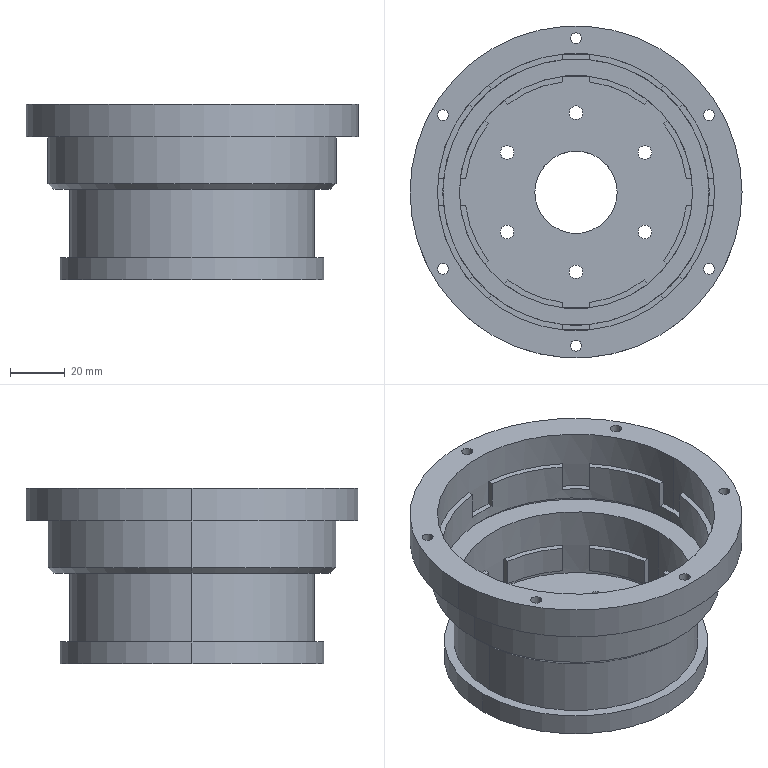Part | SolidWorks | features ICE 4, Chamfer 1, CirPattern 1, Revolution 1 | 1 solid | 124 faces | box 121 x 121 x 64.094 mm | volume 133004 mm3 | plane 72 | cylinder 50 | cone 2 | commonest cylinder face diameters 4 x12 5 x12 81 x8 101 x4 30 x2 85 x2